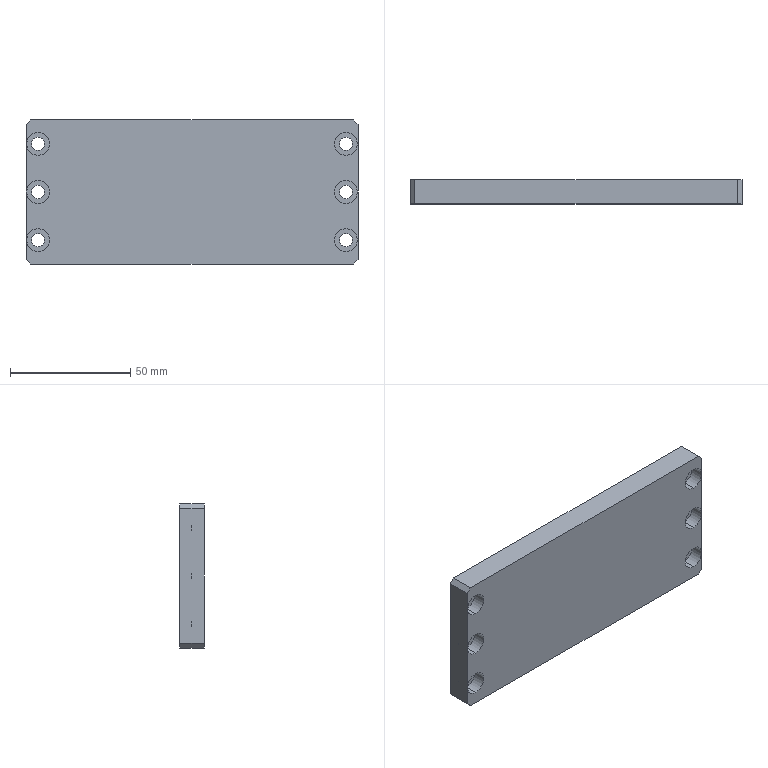Part | SolidWorks | features BaseBody 1 | 1 solid | 40 faces | box 138 x 10 x 60 mm | volume 79768 mm3 | cylinder 24 | plane 16 | commonest cylinder face diameters 5.5 x12 9.5 x12
STEP:
#1=CARTESIAN_POINT('',(-64.,5.4,-15.25));
#2=VERTEX_POINT('',#1);
#3=CARTESIAN_POINT('',(-64.,5.4,-24.75));
#4=VERTEX_POINT('',#3);
#5=CARTESIAN_POINT('',(-64.,5.4,-20.));
#6=DIRECTION('',(0.,-1.,0.));
#7=DIRECTION('',(0.,0.,-1.));
#8=AXIS2_PLACEMENT_3D('',#5,#6,#7);
#9=CIRCLE('',#8,4.75);
#10=EDGE_CURVE('',#2,#4,#9,.T.);
#11=ORIENTED_EDGE('',*,*,#10,.F.);
#12=CARTESIAN_POINT('',(-64.,0.,-15.25));
#13=VERTEX_POINT('',#12);
#14=CARTESIAN_POINT('',(-64.,0.,-15.25));
#15=DIRECTION('',(0.,-1.,0.));
#16=VECTOR('',#15,1000.);
#17=LINE('',#14,#16);
#18=EDGE_CURVE('',#2,#13,#17,.T.);
#19=ORIENTED_EDGE('',*,*,#18,.T.);
#20=CARTESIAN_POINT('',(-64.,0.,-24.75));
#21=VERTEX_POINT('',#20);
#22=CARTESIAN_POINT('',(-64.,0.,-20.));
#23=DIRECTION('',(0.,-1.,0.));
#24=DIRECTION('',(0.,0.,-1.));
#25=AXIS2_PLACEMENT_3D('',#22,#23,#24);
#26=CIRCLE('',#25,4.75);
#27=EDGE_CURVE('',#13,#21,#26,.T.);
#28=ORIENTED_EDGE('',*,*,#27,.T.);
#29=CARTESIAN_POINT('',(-64.,0.,-24.75));
#30=DIRECTION('',(0.,-1.,0.));
#31=VECTOR('',#30,1000.);
#32=LINE('',#29,#31);
#33=EDGE_CURVE('',#4,#21,#32,.T.);
#34=ORIENTED_EDGE('',*,*,#33,.F.);
#35=EDGE_LOOP('',(#11,#19,#28,#34));
#36=FACE_OUTER_BOUND('',#35,.T.);
#37=CARTESIAN_POINT('',(-64.,0.,-20.));
#38=DIRECTION('',(0.,-1.,0.));
#39=DIRECTION('',(0.,0.,-1.));
#40=AXIS2_PLACEMENT_3D('',#37,#38,#39);
#41=CYLINDRICAL_SURFACE('',#40,4.75);
#42=ADVANCED_FACE('',(#36),#41,.F.);
#43=CARTESIAN_POINT('',(-64.,10.,-17.25));
#44=VERTEX_POINT('',#43);
#45=CARTESIAN_POINT('',(-64.,10.,-22.75));
#46=VERTEX_POINT('',#45);
#47=CARTESIAN_POINT('',(-64.,10.,-20.));
#48=DIRECTION('',(0.,-1.,0.));
#49=DIRECTION('',(0.,0.,-1.));
#50=AXIS2_PLACEMENT_3D('',#47,#48,#49);
#51=CIRCLE('',#50,2.75);
#52=EDGE_CURVE('',#44,#46,#51,.T.);
#53=ORIENTED_EDGE('',*,*,#52,.F.);
#54=CARTESIAN_POINT('',(-64.,5.4,-17.25));
#55=VERTEX_POINT('',#54);
#56=CARTESIAN_POINT('',(-64.,0.,-17.25));
#57=DIRECTION('',(0.,-1.,0.));
#58=VECTOR('',#57,1000.);
#59=LINE('',#56,#58);
#60=EDGE_CURVE('',#44,#55,#59,.T.);
#61=ORIENTED_EDGE('',*,*,#60,.T.);
#62=CARTESIAN_POINT('',(-64.,5.4,-22.75));
#63=VERTEX_POINT('',#62);
#64=CARTESIAN_POINT('',(-64.,5.4,-20.));
#65=DIRECTION('',(0.,-1.,0.));
#66=DIRECTION('',(0.,0.,-1.));
#67=AXIS2_PLACEMENT_3D('',#64,#65,#66);
#68=CIRCLE('',#67,2.75);
#69=EDGE_CURVE('',#55,#63,#68,.T.);
#70=ORIENTED_EDGE('',*,*,#69,.T.);
#71=CARTESIAN_POINT('',(-64.,0.,-22.75));
#72=DIRECTION('',(0.,-1.,0.));
#73=VECTOR('',#72,1000.);
#74=LINE('',#71,#73);
#75=EDGE_CURVE('',#46,#63,#74,.T.);
#76=ORIENTED_EDGE('',*,*,#75,.F.);
#77=EDGE_LOOP('',(#53,#61,#70,#76));
#78=FACE_OUTER_BOUND('',#77,.T.);
#79=CARTESIAN_POINT('',(-64.,0.,-20.));
#80=DIRECTION('',(0.,-1.,0.));
#81=DIRECTION('',(0.,0.,-1.));
#82=AXIS2_PLACEMENT_3D('',#79,#80,#81);
#83=CYLINDRICAL_SURFACE('',#82,2.75);
#84=ADVANCED_FACE('',(#78),#83,.F.);
#85=CARTESIAN_POINT('',(-64.,5.4,4.75));
#86=VERTEX_POINT('',#85);
#87=CARTESIAN_POINT('',(-64.,5.4,-4.75));
#88=VERTEX_POINT('',#87);
#89=CARTESIAN_POINT('',(-64.,5.4,0.));
#90=DIRECTION('',(0.,-1.,0.));
#91=DIRECTION('',(0.,0.,-1.));
#92=AXIS2_PLACEMENT_3D('',#89,#90,#91);
#93=CIRCLE('',#92,4.75);
#94=EDGE_CURVE('',#86,#88,#93,.T.);
#95=ORIENTED_EDGE('',*,*,#94,.F.);
#96=CARTESIAN_POINT('',(-64.,0.,4.75));
#97=VERTEX_POINT('',#96);
#98=CARTESIAN_POINT('',(-64.,0.,4.75));
#99=DIRECTION('',(0.,-1.,0.));
#100=VECTOR('',#99,1000.);
#101=LINE('',#98,#100);
#102=EDGE_CURVE('',#86,#97,#101,.T.);
#103=ORIENTED_EDGE('',*,*,#102,.T.);
#104=CARTESIAN_POINT('',(-64.,0.,-4.75));
#105=VERTEX_POINT('',#104);
#106=CARTESIAN_POINT('',(-64.,0.,0.));
#107=DIRECTION('',(0.,-1.,0.));
#108=DIRECTION('',(0.,0.,-1.));
#109=AXIS2_PLACEMENT_3D('',#106,#107,#108);
#110=CIRCLE('',#109,4.75);
#111=EDGE_CURVE('',#97,#105,#110,.T.);
#112=ORIENTED_EDGE('',*,*,#111,.T.);
#113=CARTESIAN_POINT('',(-64.,0.,-4.75));
#114=DIRECTION('',(0.,-1.,0.));
#115=VECTOR('',#114,1000.);
#116=LINE('',#113,#115);
#117=EDGE_CURVE('',#88,#105,#116,.T.);
#118=ORIENTED_EDGE('',*,*,#117,.F.);
#119=EDGE_LOOP('',(#95,#103,#112,#118));
#120=FACE_OUTER_BOUND('',#119,.T.);
#121=CARTESIAN_POINT('',(-64.,0.,0.));
#122=DIRECTION('',(0.,-1.,0.));
#123=DIRECTION('',(0.,0.,-1.));
#124=AXIS2_PLACEMENT_3D('',#121,#122,#123);
#125=CYLINDRICAL_SURFACE('',#124,4.75);
#126=ADVANCED_FACE('',(#120),#125,.F.);
#127=CARTESIAN_POINT('',(-64.,10.,2.75));
#128=VERTEX_POINT('',#127);
#129=CARTESIAN_POINT('',(-64.,10.,-2.75));
#130=VERTEX_POINT('',#129);
#131=CARTESIAN_POINT('',(-64.,10.,0.));
#132=DIRECTION('',(0.,-1.,0.));
#133=DIRECTION('',(0.,0.,-1.));
#134=AXIS2_PLACEMENT_3D('',#131,#132,#133);
#135=CIRCLE('',#134,2.75);
#136=EDGE_CURVE('',#128,#130,#135,.T.);
#137=ORIENTED_EDGE('',*,*,#136,.F.);
#138=CARTESIAN_POINT('',(-64.,5.4,2.75));
#139=VERTEX_POINT('',#138);
#140=CARTESIAN_POINT('',(-64.,0.,2.75));
#141=DIRECTION('',(0.,-1.,0.));
#142=VECTOR('',#141,1000.);
#143=LINE('',#140,#142);
#144=EDGE_CURVE('',#128,#139,#143,.T.);
#145=ORIENTED_EDGE('',*,*,#144,.T.);
#146=CARTESIAN_POINT('',(-64.,5.4,-2.75));
#147=VERTEX_POINT('',#146);
#148=CARTESIAN_POINT('',(-64.,5.4,0.));
#149=DIRECTION('',(0.,-1.,0.));
#150=DIRECTION('',(0.,0.,-1.));
#151=AXIS2_PLACEMENT_3D('',#148,#149,#150);
#152=CIRCLE('',#151,2.75);
#153=EDGE_CURVE('',#139,#147,#152,.T.);
#154=ORIENTED_EDGE('',*,*,#153,.T.);
#155=CARTESIAN_POINT('',(-64.,0.,-2.75));
#156=DIRECTION('',(0.,-1.,0.));
#157=VECTOR('',#156,1000.);
#158=LINE('',#155,#157);
#159=EDGE_CURVE('',#130,#147,#158,.T.);
#160=ORIENTED_EDGE('',*,*,#159,.F.);
#161=EDGE_LOOP('',(#137,#145,#154,#160));
#162=FACE_OUTER_BOUND('',#161,.T.);
#163=CARTESIAN_POINT('',(-64.,0.,0.));
#164=DIRECTION('',(0.,-1.,0.));
#165=DIRECTION('',(0.,0.,-1.));
#166=AXIS2_PLACEMENT_3D('',#163,#164,#165);
#167=CYLINDRICAL_SURFACE('',#166,2.75);
#168=ADVANCED_FACE('',(#162),#167,.F.);
#169=CARTESIAN_POINT('',(-64.,5.4,24.75));
#170=VERTEX_POINT('',#169);
#171=CARTESIAN_POINT('',(-64.,5.4,15.25));
#172=VERTEX_POINT('',#171);
#173=CARTESIAN_POINT('',(-64.,5.4,20.));
#174=DIRECTION('',(0.,-1.,0.));
#175=DIRECTION('',(0.,0.,-1.));
#176=AXIS2_PLACEMENT_3D('',#173,#174,#175);
#177=CIRCLE('',#176,4.75);
#178=EDGE_CURVE('',#170,#172,#177,.T.);
#179=ORIENTED_EDGE('',*,*,#178,.F.);
#180=CARTESIAN_POINT('',(-64.,0.,24.75));
#181=VERTEX_POINT('',#180);
#182=CARTESIAN_POINT('',(-64.,0.,24.75));
#183=DIRECTION('',(0.,-1.,0.));
#184=VECTOR('',#183,1000.);
#185=LINE('',#182,#184);
#186=EDGE_CURVE('',#170,#181,#185,.T.);
#187=ORIENTED_EDGE('',*,*,#186,.T.);
#188=CARTESIAN_POINT('',(-64.,0.,15.25));
#189=VERTEX_POINT('',#188);
#190=CARTESIAN_POINT('',(-64.,0.,20.));
#191=DIRECTION('',(0.,-1.,0.));
#192=DIRECTION('',(0.,0.,-1.));
#193=AXIS2_PLACEMENT_3D('',#190,#191,#192);
#194=CIRCLE('',#193,4.75);
#195=EDGE_CURVE('',#181,#189,#194,.T.);
#196=ORIENTED_EDGE('',*,*,#195,.T.);
#197=CARTESIAN_POINT('',(-64.,0.,15.25));
#198=DIRECTION('',(0.,-1.,0.));
#199=VECTOR('',#198,1000.);
#200=LINE('',#197,#199);
#201=EDGE_CURVE('',#172,#189,#200,.T.);
#202=ORIENTED_EDGE('',*,*,#201,.F.);
#203=EDGE_LOOP('',(#179,#187,#196,#202));
#204=FACE_OUTER_BOUND('',#203,.T.);
#205=CARTESIAN_POINT('',(-64.,0.,20.));
#206=DIRECTION('',(0.,-1.,0.));
#207=DIRECTION('',(0.,0.,-1.));
#208=AXIS2_PLACEMENT_3D('',#205,#206,#207);
#209=CYLINDRICAL_SURFACE('',#208,4.75);
#210=ADVANCED_FACE('',(#204),#209,.F.);
#211=CARTESIAN_POINT('',(-64.,10.,22.75));
#212=VERTEX_POINT('',#211);
#213=CARTESIAN_POINT('',(-64.,10.,17.25));
#214=VERTEX_POINT('',#213);
#215=CARTESIAN_POINT('',(-64.,10.,20.));
#216=DIRECTION('',(0.,-1.,0.));
#217=DIRECTION('',(0.,0.,-1.));
#218=AXIS2_PLACEMENT_3D('',#215,#216,#217);
#219=CIRCLE('',#218,2.75);
#220=EDGE_CURVE('',#212,#214,#219,.T.);
#221=ORIENTED_EDGE('',*,*,#220,.F.);
#222=CARTESIAN_POINT('',(-64.,5.4,22.75));
#223=VERTEX_POINT('',#222);
#224=CARTESIAN_POINT('',(-64.,0.,22.75));
#225=DIRECTION('',(0.,-1.,0.));
#226=VECTOR('',#225,1000.);
#227=LINE('',#224,#226);
#228=EDGE_CURVE('',#212,#223,#227,.T.);
#229=ORIENTED_EDGE('',*,*,#228,.T.);
#230=CARTESIAN_POINT('',(-64.,5.4,17.25));
#231=VERTEX_POINT('',#230);
#232=CARTESIAN_POINT('',(-64.,5.4,20.));
#233=DIRECTION('',(0.,-1.,0.));
#234=DIRECTION('',(0.,0.,-1.));
#235=AXIS2_PLACEMENT_3D('',#232,#233,#234);
#236=CIRCLE('',#235,2.75);
#237=EDGE_CURVE('',#223,#231,#236,.T.);
#238=ORIENTED_EDGE('',*,*,#237,.T.);
#239=CARTESIAN_POINT('',(-64.,0.,17.25));
#240=DIRECTION('',(0.,-1.,0.));
#241=VECTOR('',#240,1000.);
#242=LINE('',#239,#241);
#243=EDGE_CURVE('',#214,#231,#242,.T.);
#244=ORIENTED_EDGE('',*,*,#243,.F.);
#245=EDGE_LOOP('',(#221,#229,#238,#244));
#246=FACE_OUTER_BOUND('',#245,.T.);
#247=CARTESIAN_POINT('',(-64.,0.,20.));
#248=DIRECTION('',(0.,-1.,0.));
#249=DIRECTION('',(0.,0.,-1.));
#250=AXIS2_PLACEMENT_3D('',#247,#248,#249);
#251=CYLINDRICAL_SURFACE('',#250,2.75);
#252=ADVANCED_FACE('',(#246),#251,.F.);
#253=CARTESIAN_POINT('',(64.,5.4,24.75));
#254=VERTEX_POINT('',#253);
#255=CARTESIAN_POINT('',(64.,5.4,15.25));
#256=VERTEX_POINT('',#255);
#257=CARTESIAN_POINT('',(64.,5.4,20.));
#258=DIRECTION('',(0.,-1.,0.));
#259=DIRECTION('',(0.,0.,-1.));
#260=AXIS2_PLACEMENT_3D('',#257,#258,#259);
#261=CIRCLE('',#260,4.75);
#262=EDGE_CURVE('',#254,#256,#261,.T.);
#263=ORIENTED_EDGE('',*,*,#262,.F.);
#264=CARTESIAN_POINT('',(64.,0.,24.75));
#265=VERTEX_POINT('',#264);
#266=CARTESIAN_POINT('',(64.,0.,24.75));
#267=DIRECTION('',(0.,-1.,0.));
#268=VECTOR('',#267,1000.);
#269=LINE('',#266,#268);
#270=EDGE_CURVE('',#254,#265,#269,.T.);
#271=ORIENTED_EDGE('',*,*,#270,.T.);
#272=CARTESIAN_POINT('',(64.,0.,15.25));
#273=VERTEX_POINT('',#272);
#274=CARTESIAN_POINT('',(64.,0.,20.));
#275=DIRECTION('',(0.,-1.,0.));
#276=DIRECTION('',(0.,0.,-1.));
#277=AXIS2_PLACEMENT_3D('',#274,#275,#276);
#278=CIRCLE('',#277,4.75);
#279=EDGE_CURVE('',#265,#273,#278,.T.);
#280=ORIENTED_EDGE('',*,*,#279,.T.);
#281=CARTESIAN_POINT('',(64.,0.,15.25));
#282=DIRECTION('',(0.,-1.,0.));
#283=VECTOR('',#282,1000.);
#284=LINE('',#281,#283);
#285=EDGE_CURVE('',#256,#273,#284,.T.);
#286=ORIENTED_EDGE('',*,*,#285,.F.);
#287=EDGE_LOOP('',(#263,#271,#280,#286));
#288=FACE_OUTER_BOUND('',#287,.T.);
#289=CARTESIAN_POINT('',(64.,0.,20.));
#290=DIRECTION('',(0.,-1.,0.));
#291=DIRECTION('',(0.,0.,-1.));
#292=AXIS2_PLACEMENT_3D('',#289,#290,#291);
#293=CYLINDRICAL_SURFACE('',#292,4.75);
#294=ADVANCED_FACE('',(#288),#293,.F.);
#295=CARTESIAN_POINT('',(64.,10.,22.75));
#296=VERTEX_POINT('',#295);
#297=CARTESIAN_POINT('',(64.,10.,17.25));
#298=VERTEX_POINT('',#297);
#299=CARTESIAN_POINT('',(64.,10.,20.));
#300=DIRECTION('',(0.,-1.,0.));
#301=DIRECTION('',(0.,0.,-1.));
#302=AXIS2_PLACEMENT_3D('',#299,#300,#301);
#303=CIRCLE('',#302,2.75);
#304=EDGE_CURVE('',#296,#298,#303,.T.);
#305=ORIENTED_EDGE('',*,*,#304,.F.);
#306=CARTESIAN_POINT('',(64.,5.4,22.75));
#307=VERTEX_POINT('',#306);
#308=CARTESIAN_POINT('',(64.,0.,22.75));
#309=DIRECTION('',(0.,-1.,0.));
#310=VECTOR('',#309,1000.);
#311=LINE('',#308,#310);
#312=EDGE_CURVE('',#296,#307,#311,.T.);
#313=ORIENTED_EDGE('',*,*,#312,.T.);
#314=CARTESIAN_POINT('',(64.,5.4,17.25));
#315=VERTEX_POINT('',#314);
#316=CARTESIAN_POINT('',(64.,5.4,20.));
#317=DIRECTION('',(0.,-1.,0.));
#318=DIRECTION('',(0.,0.,-1.));
#319=AXIS2_PLACEMENT_3D('',#316,#317,#318);
#320=CIRCLE('',#319,2.75);
#321=EDGE_CURVE('',#307,#315,#320,.T.);
#322=ORIENTED_EDGE('',*,*,#321,.T.);
#323=CARTESIAN_POINT('',(64.,0.,17.25));
#324=DIRECTION('',(0.,-1.,0.));
#325=VECTOR('',#324,1000.);
#326=LINE('',#323,#325);
#327=EDGE_CURVE('',#298,#315,#326,.T.);
#328=ORIENTED_EDGE('',*,*,#327,.F.);
#329=EDGE_LOOP('',(#305,#313,#322,#328));
#330=FACE_OUTER_BOUND('',#329,.T.);
#331=CARTESIAN_POINT('',(64.,0.,20.));
#332=DIRECTION('',(0.,-1.,0.));
#333=DIRECTION('',(0.,0.,-1.));
#334=AXIS2_PLACEMENT_3D('',#331,#332,#333);
#335=CYLINDRICAL_SURFACE('',#334,2.75);
#336=ADVANCED_FACE('',(#330),#335,.F.);
#337=CARTESIAN_POINT('',(64.,5.4,4.75));
#338=VERTEX_POINT('',#337);
#339=CARTESIAN_POINT('',(64.,5.4,-4.75));
#340=VERTEX_POINT('',#339);
#341=CARTESIAN_POINT('',(64.,5.4,0.));
#342=DIRECTION('',(0.,-1.,0.));
#343=DIRECTION('',(0.,0.,-1.));
#344=AXIS2_PLACEMENT_3D('',#341,#342,#343);
#345=CIRCLE('',#344,4.75);
#346=EDGE_CURVE('',#338,#340,#345,.T.);
#347=ORIENTED_EDGE('',*,*,#346,.F.);
#348=CARTESIAN_POINT('',(64.,0.,4.75));
#349=VERTEX_POINT('',#348);
#350=CARTESIAN_POINT('',(64.,0.,4.75));
#351=DIRECTION('',(0.,-1.,0.));
#352=VECTOR('',#351,1000.);
#353=LINE('',#350,#352);
#354=EDGE_CURVE('',#338,#349,#353,.T.);
#355=ORIENTED_EDGE('',*,*,#354,.T.);
#356=CARTESIAN_POINT('',(64.,0.,-4.75));
#357=VERTEX_POINT('',#356);
#358=CARTESIAN_POINT('',(64.,0.,0.));
#359=DIRECTION('',(0.,-1.,0.));
#360=DIRECTION('',(0.,0.,-1.));
#361=AXIS2_PLACEMENT_3D('',#358,#359,#360);
#362=CIRCLE('',#361,4.75);
#363=EDGE_CURVE('',#349,#357,#362,.T.);
#364=ORIENTED_EDGE('',*,*,#363,.T.);
#365=CARTESIAN_POINT('',(64.,0.,-4.75));
#366=DIRECTION('',(0.,-1.,0.));
#367=VECTOR('',#366,1000.);
#368=LINE('',#365,#367);
#369=EDGE_CURVE('',#340,#357,#368,.T.);
#370=ORIENTED_EDGE('',*,*,#369,.F.);
#371=EDGE_LOOP('',(#347,#355,#364,#370));
#372=FACE_OUTER_BOUND('',#371,.T.);
#373=CARTESIAN_POINT('',(64.,0.,0.));
#374=DIRECTION('',(0.,-1.,0.));
#375=DIRECTION('',(0.,0.,-1.));
#376=AXIS2_PLACEMENT_3D('',#373,#374,#375);
#377=CYLINDRICAL_SURFACE('',#376,4.75);
#378=ADVANCED_FACE('',(#372),#377,.F.);
#379=CARTESIAN_POINT('',(64.,10.,2.75));
#380=VERTEX_POINT('',#379);
#381=CARTESIAN_POINT('',(64.,10.,-2.75));
#382=VERTEX_POINT('',#381);
#383=CARTESIAN_POINT('',(64.,10.,0.));
#384=DIRECTION('',(0.,-1.,0.));
#385=DIRECTION('',(0.,0.,-1.));
#386=AXIS2_PLACEMENT_3D('',#383,#384,#385);
#387=CIRCLE('',#386,2.75);
#388=EDGE_CURVE('',#380,#382,#387,.T.);
#389=ORIENTED_EDGE('',*,*,#388,.F.);
#390=CARTESIAN_POINT('',(64.,5.4,2.75));
#391=VERTEX_POINT('',#390);
#392=CARTESIAN_POINT('',(64.,0.,2.75));
#393=DIRECTION('',(0.,-1.,0.));
#394=VECTOR('',#393,1000.);
#395=LINE('',#392,#394);
#396=EDGE_CURVE('',#380,#391,#395,.T.);
#397=ORIENTED_EDGE('',*,*,#396,.T.);
#398=CARTESIAN_POINT('',(64.,5.4,-2.75));
#399=VERTEX_POINT('',#398);
#400=CARTESIAN_POINT('',(64.,5.4,0.));
#401=DIRECTION('',(0.,-1.,0.));
#402=DIRECTION('',(0.,0.,-1.));
#403=AXIS2_PLACEMENT_3D('',#400,#401,#402);
#404=CIRCLE('',#403,2.75);
#405=EDGE_CURVE('',#391,#399,#404,.T.);
#406=ORIENTED_EDGE('',*,*,#405,.T.);
#407=CARTESIAN_POINT('',(64.,0.,-2.75));
#408=DIRECTION('',(0.,-1.,0.));
#409=VECTOR('',#408,1000.);
#410=LINE('',#407,#409);
#411=EDGE_CURVE('',#382,#399,#410,.T.);
#412=ORIENTED_EDGE('',*,*,#411,.F.);
#413=EDGE_LOOP('',(#389,#397,#406,#412));
#414=FACE_OUTER_BOUND('',#413,.T.);
#415=CARTESIAN_POINT('',(64.,0.,0.));
#416=DIRECTION('',(0.,-1.,0.));
#417=DIRECTION('',(0.,0.,-1.));
#418=AXIS2_PLACEMENT_3D('',#415,#416,#417);
#419=CYLINDRICAL_SURFACE('',#418,2.75);
#420=ADVANCED_FACE('',(#414),#419,.F.);
#421=CARTESIAN_POINT('',(64.,5.4,-15.25));
#422=VERTEX_POINT('',#421);
#423=CARTESIAN_POINT('',(64.,5.4,-24.75));
#424=VERTEX_POINT('',#423);
#425=CARTESIAN_POINT('',(64.,5.4,-20.));
#426=DIRECTION('',(0.,-1.,0.));
#427=DIRECTION('',(0.,0.,-1.));
#428=AXIS2_PLACEMENT_3D('',#425,#426,#427);
#429=CIRCLE('',#428,4.75);
#430=EDGE_CURVE('',#422,#424,#429,.T.);
#431=ORIENTED_EDGE('',*,*,#430,.F.);
#432=CARTESIAN_POINT('',(64.,0.,-15.25));
#433=VERTEX_POINT('',#432);
#434=CARTESIAN_POINT('',(64.,0.,-15.25));
#435=DIRECTION('',(0.,-1.,0.));
#436=VECTOR('',#435,1000.);
#437=LINE('',#434,#436);
#438=EDGE_CURVE('',#422,#433,#437,.T.);
#439=ORIENTED_EDGE('',*,*,#438,.T.);
#440=CARTESIAN_POINT('',(64.,0.,-24.75));
#441=VERTEX_POINT('',#440);
#442=CARTESIAN_POINT('',(64.,0.,-20.));
#443=DIRECTION('',(0.,-1.,0.));
#444=DIRECTION('',(0.,0.,-1.));
#445=AXIS2_PLACEMENT_3D('',#442,#443,#444);
#446=CIRCLE('',#445,4.75);
#447=EDGE_CURVE('',#433,#441,#446,.T.);
#448=ORIENTED_EDGE('',*,*,#447,.T.);
#449=CARTESIAN_POINT('',(64.,0.,-24.75));
#450=DIRECTION('',(0.,-1.,0.));
#451=VECTOR('',#450,1000.);
#452=LINE('',#449,#451);
#453=EDGE_CURVE('',#424,#441,#452,.T.);
#454=ORIENTED_EDGE('',*,*,#453,.F.);
#455=EDGE_LOOP('',(#431,#439,#448,#454));
#456=FACE_OUTER_BOUND('',#455,.T.);
#457=CARTESIAN_POINT('',(64.,0.,-20.));
#458=DIRECTION('',(0.,-1.,0.));
#459=DIRECTION('',(0.,0.,-1.));
#460=AXIS2_PLACEMENT_3D('',#457,#458,#459);
#461=CYLINDRICAL_SURFACE('',#460,4.75);
#462=ADVANCED_FACE('',(#456),#461,.F.);
#463=CARTESIAN_POINT('',(64.,10.,-17.25));
#464=VERTEX_POINT('',#463);
#465=CARTESIAN_POINT('',(64.,10.,-22.75));
#466=VERTEX_POINT('',#465);
#467=CARTESIAN_POINT('',(64.,10.,-20.));
#468=DIRECTION('',(0.,-1.,0.));
#469=DIRECTION('',(0.,0.,-1.));
#470=AXIS2_PLACEMENT_3D('',#467,#468,#469);
#471=CIRCLE('',#470,2.75);
#472=EDGE_CURVE('',#464,#466,#471,.T.);
#473=ORIENTED_EDGE('',*,*,#472,.F.);
#474=CARTESIAN_POINT('',(64.,5.4,-17.25));
#475=VERTEX_POINT('',#474);
#476=CARTESIAN_POINT('',(64.,0.,-17.25));
#477=DIRECTION('',(0.,-1.,0.));
#478=VECTOR('',#477,1000.);
#479=LINE('',#476,#478);
#480=EDGE_CURVE('',#464,#475,#479,.T.);
#481=ORIENTED_EDGE('',*,*,#480,.T.);
#482=CARTESIAN_POINT('',(64.,5.4,-22.75));
#483=VERTEX_POINT('',#482);
#484=CARTESIAN_POINT('',(64.,5.4,-20.));
#485=DIRECTION('',(0.,-1.,0.));
#486=DIRECTION('',(0.,0.,-1.));
#487=AXIS2_PLACEMENT_3D('',#484,#485,#486);
#488=CIRCLE('',#487,2.75);
#489=EDGE_CURVE('',#475,#483,#488,.T.);
#490=ORIENTED_EDGE('',*,*,#489,.T.);
#491=CARTESIAN_POINT('',(64.,0.,-22.75));
#492=DIRECTION('',(0.,-1.,0.));
#493=VECTOR('',#492,1000.);
#494=LINE('',#491,#493);
#495=EDGE_CURVE('',#466,#483,#494,.T.);
#496=ORIENTED_EDGE('',*,*,#495,.F.);
#497=EDGE_LOOP('',(#473,#481,#490,#496));
#498=FACE_OUTER_BOUND('',#497,.T.);
#499=CARTESIAN_POINT('',(64.,0.,-20.));
#500=DIRECTION('',(0.,-1.,0.));
#501=DIRECTION('',(0.,0.,-1.));
#502=AXIS2_PLACEMENT_3D('',#499,#500,#501);
#503=CYLINDRICAL_SURFACE('',#502,2.75);
#504=ADVANCED_FACE('',(#498),#503,.F.);
#505=CARTESIAN_POINT('',(-69.,10.,-28.));
#506=VERTEX_POINT('',#505);
#507=CARTESIAN_POINT('',(-69.,10.,28.));
#508=VERTEX_POINT('',#507);
#509=CARTESIAN_POINT('',(-69.,10.,-30.));
#510=DIRECTION('',(0.,0.,1.));
#511=VECTOR('',#510,1000.);
#512=LINE('',#509,#511);
#513=EDGE_CURVE('',#506,#508,#512,.T.);
#514=ORIENTED_EDGE('',*,*,#513,.F.);
#515=CARTESIAN_POINT('',(-69.,0.,-28.));
#516=VERTEX_POINT('',#515);
#517=CARTESIAN_POINT('',(-69.,10.,-28.));
#518=DIRECTION('',(0.,-1.,0.));
#519=VECTOR('',#518,1000.);
#520=LINE('',#517,#519);
#521=EDGE_CURVE('',#506,#516,#520,.T.);
#522=ORIENTED_EDGE('',*,*,#521,.T.);
#523=CARTESIAN_POINT('',(-69.,0.,28.));
#524=VERTEX_POINT('',#523);
#525=CARTESIAN_POINT('',(-69.,0.,-30.));
#526=DIRECTION('',(0.,0.,1.));
#527=VECTOR('',#526,1000.);
#528=LINE('',#525,#527);
#529=EDGE_CURVE('',#516,#524,#528,.T.);
#530=ORIENTED_EDGE('',*,*,#529,.T.);
#531=CARTESIAN_POINT('',(-69.,10.,28.));
#532=DIRECTION('',(0.,1.,0.));
#533=VECTOR('',#532,1000.);
#534=LINE('',#531,#533);
#535=EDGE_CURVE('',#524,#508,#534,.T.);
#536=ORIENTED_EDGE('',*,*,#535,.T.);
#537=EDGE_LOOP('',(#514,#522,#530,#536));
#538=FACE_OUTER_BOUND('',#537,.T.);
#539=CARTESIAN_POINT('',(-69.,10.,-30.));
#540=DIRECTION('',(1.,0.,0.));
#541=DIRECTION('',(0.,0.,-1.));
#542=AXIS2_PLACEMENT_3D('',#539,#540,#541);
#543=PLANE('',#542);
#544=ADVANCED_FACE('',(#538),#543,.F.);
#545=CARTESIAN_POINT('',(-67.,0.,30.));
#546=VERTEX_POINT('',#545);
#547=CARTESIAN_POINT('',(67.,0.,30.));
#548=VERTEX_POINT('',#547);
#549=CARTESIAN_POINT('',(69.,0.,30.));
#550=DIRECTION('',(1.,0.,0.));
#551=VECTOR('',#550,1000.);
#552=LINE('',#549,#551);
#553=EDGE_CURVE('',#546,#548,#552,.T.);
#554=ORIENTED_EDGE('',*,*,#553,.T.);
#555=CARTESIAN_POINT('',(67.,10.,30.));
#556=VERTEX_POINT('',#555);
#557=CARTESIAN_POINT('',(67.,10.,30.));
#558=DIRECTION('',(0.,1.,0.));
#559=VECTOR('',#558,1000.);
#560=LINE('',#557,#559);
#561=EDGE_CURVE('',#548,#556,#560,.T.);
#562=ORIENTED_EDGE('',*,*,#561,.T.);
#563=CARTESIAN_POINT('',(-67.,10.,30.));
#564=VERTEX_POINT('',#563);
#565=CARTESIAN_POINT('',(69.,10.,30.));
#566=DIRECTION('',(1.,0.,0.));
#567=VECTOR('',#566,1000.);
#568=LINE('',#565,#567);
#569=EDGE_CURVE('',#564,#556,#568,.T.);
#570=ORIENTED_EDGE('',*,*,#569,.F.);
#571=CARTESIAN_POINT('',(-67.,10.,30.));
#572=DIRECTION('',(0.,-1.,0.));
#573=VECTOR('',#572,1000.);
#574=LINE('',#571,#573);
#575=EDGE_CURVE('',#564,#546,#574,.T.);
#576=ORIENTED_EDGE('',*,*,#575,.T.);
#577=EDGE_LOOP('',(#554,#562,#570,#576));
#578=FACE_OUTER_BOUND('',#577,.T.);
#579=CARTESIAN_POINT('',(69.,10.,30.));
#580=DIRECTION('',(0.,0.,-1.));
#581=DIRECTION('',(-1.,0.,0.));
#582=AXIS2_PLACEMENT_3D('',#579,#580,#581);
#583=PLANE('',#582);
#584=ADVANCED_FACE('',(#578),#583,.F.);
#585=CARTESIAN_POINT('',(69.,10.,28.));
#586=VERTEX_POINT('',#585);
#587=CARTESIAN_POINT('',(69.,10.,-28.));
#588=VERTEX_POINT('',#587);
#589=CARTESIAN_POINT('',(69.,10.,-30.));
#590=DIRECTION('',(0.,0.,-1.));
#591=VECTOR('',#590,1000.);
#592=LINE('',#589,#591);
#593=EDGE_CURVE('',#586,#588,#592,.T.);
#594=ORIENTED_EDGE('',*,*,#593,.F.);
#595=CARTESIAN_POINT('',(69.,0.,28.));
#596=VERTEX_POINT('',#595);
#597=CARTESIAN_POINT('',(69.,10.,28.));
#598=DIRECTION('',(0.,-1.,0.));
#599=VECTOR('',#598,1000.);
#600=LINE('',#597,#599);
#601=EDGE_CURVE('',#586,#596,#600,.T.);
#602=ORIENTED_EDGE('',*,*,#601,.T.);
#603=CARTESIAN_POINT('',(69.,0.,-28.));
#604=VERTEX_POINT('',#603);
#605=CARTESIAN_POINT('',(69.,0.,-30.));
#606=DIRECTION('',(0.,0.,-1.));
#607=VECTOR('',#606,1000.);
#608=LINE('',#605,#607);
#609=EDGE_CURVE('',#596,#604,#608,.T.);
#610=ORIENTED_EDGE('',*,*,#609,.T.);
#611=CARTESIAN_POINT('',(69.,10.,-28.));
#612=DIRECTION('',(0.,1.,0.));
#613=VECTOR('',#612,1000.);
#614=LINE('',#611,#613);
#615=EDGE_CURVE('',#604,#588,#614,.T.);
#616=ORIENTED_EDGE('',*,*,#615,.T.);
#617=EDGE_LOOP('',(#594,#602,#610,#616));
#618=FACE_OUTER_BOUND('',#617,.T.);
#619=CARTESIAN_POINT('',(69.,10.,-30.));
#620=DIRECTION('',(-1.,0.,0.));
#621=DIRECTION('',(0.,0.,1.));
#622=AXIS2_PLACEMENT_3D('',#619,#620,#621);
#623=PLANE('',#622);
#624=ADVANCED_FACE('',(#618),#623,.F.);
#625=CARTESIAN_POINT('',(67.,10.,-30.));
#626=VERTEX_POINT('',#625);
#627=CARTESIAN_POINT('',(-67.,10.,-30.));
#628=VERTEX_POINT('',#627);
#629=CARTESIAN_POINT('',(69.,10.,-30.));
#630=DIRECTION('',(-1.,0.,0.));
#631=VECTOR('',#630,1000.);
#632=LINE('',#629,#631);
#633=EDGE_CURVE('',#626,#628,#632,.T.);
#634=ORIENTED_EDGE('',*,*,#633,.F.);
#635=CARTESIAN_POINT('',(67.,0.,-30.));
#636=VERTEX_POINT('',#635);
#637=CARTESIAN_POINT('',(67.,10.,-30.));
#638=DIRECTION('',(0.,-1.,0.));
#639=VECTOR('',#638,1000.);
#640=LINE('',#637,#639);
#641=EDGE_CURVE('',#626,#636,#640,.T.);
#642=ORIENTED_EDGE('',*,*,#641,.T.);
#643=CARTESIAN_POINT('',(-67.,0.,-30.));
#644=VERTEX_POINT('',#643);
#645=CARTESIAN_POINT('',(69.,0.,-30.));
#646=DIRECTION('',(-1.,0.,0.));
#647=VECTOR('',#646,1000.);
#648=LINE('',#645,#647);
#649=EDGE_CURVE('',#636,#644,#648,.T.);
#650=ORIENTED_EDGE('',*,*,#649,.T.);
#651=CARTESIAN_POINT('',(-67.,10.,-30.));
#652=DIRECTION('',(0.,1.,0.));
#653=VECTOR('',#652,1000.);
#654=LINE('',#651,#653);
#655=EDGE_CURVE('',#644,#628,#654,.T.);
#656=ORIENTED_EDGE('',*,*,#655,.T.);
#657=EDGE_LOOP('',(#634,#642,#650,#656));
#658=FACE_OUTER_BOUND('',#657,.T.);
#659=CARTESIAN_POINT('',(69.,10.,-30.));
#660=DIRECTION('',(0.,0.,1.));
#661=DIRECTION('',(1.,0.,0.));
#662=AXIS2_PLACEMENT_3D('',#659,#660,#661);
#663=PLANE('',#662);
#664=ADVANCED_FACE('',(#658),#663,.F.);
#665=CARTESIAN_POINT('',(-64.,10.,-20.));
#666=DIRECTION('',(0.,-1.,0.));
#667=DIRECTION('',(0.,0.,-1.));
#668=AXIS2_PLACEMENT_3D('',#665,#666,#667);
#669=CIRCLE('',#668,2.75);
#670=EDGE_CURVE('',#46,#44,#669,.T.);
#671=ORIENTED_EDGE('',*,*,#670,.T.);
#672=ORIENTED_EDGE('',*,*,#52,.T.);
#673=EDGE_LOOP('',(#671,#672));
#674=FACE_BOUND('',#673,.T.);
#675=CARTESIAN_POINT('',(-64.,10.,0.));
#676=DIRECTION('',(0.,-1.,0.));
#677=DIRECTION('',(0.,0.,-1.));
#678=AXIS2_PLACEMENT_3D('',#675,#676,#677);
#679=CIRCLE('',#678,2.75);
#680=EDGE_CURVE('',#130,#128,#679,.T.);
#681=ORIENTED_EDGE('',*,*,#680,.T.);
#682=ORIENTED_EDGE('',*,*,#136,.T.);
#683=EDGE_LOOP('',(#681,#682));
#684=FACE_BOUND('',#683,.T.);
#685=CARTESIAN_POINT('',(-64.,10.,20.));
#686=DIRECTION('',(0.,-1.,0.));
#687=DIRECTION('',(0.,0.,-1.));
#688=AXIS2_PLACEMENT_3D('',#685,#686,#687);
#689=CIRCLE('',#688,2.75);
#690=EDGE_CURVE('',#214,#212,#689,.T.);
#691=ORIENTED_EDGE('',*,*,#690,.T.);
#692=ORIENTED_EDGE('',*,*,#220,.T.);
#693=EDGE_LOOP('',(#691,#692));
#694=FACE_BOUND('',#693,.T.);
#695=CARTESIAN_POINT('',(64.,10.,20.));
#696=DIRECTION('',(0.,-1.,0.));
#697=DIRECTION('',(0.,0.,-1.));
#698=AXIS2_PLACEMENT_3D('',#695,#696,#697);
#699=CIRCLE('',#698,2.75);
#700=EDGE_CURVE('',#298,#296,#699,.T.);
#701=ORIENTED_EDGE('',*,*,#700,.T.);
#702=ORIENTED_EDGE('',*,*,#304,.T.);
#703=EDGE_LOOP('',(#701,#702));
#704=FACE_BOUND('',#703,.T.);
#705=CARTESIAN_POINT('',(64.,10.,0.));
#706=DIRECTION('',(0.,-1.,0.));
#707=DIRECTION('',(0.,0.,-1.));
#708=AXIS2_PLACEMENT_3D('',#705,#706,#707);
#709=CIRCLE('',#708,2.75);
#710=EDGE_CURVE('',#382,#380,#709,.T.);
#711=ORIENTED_EDGE('',*,*,#710,.T.);
#712=ORIENTED_EDGE('',*,*,#388,.T.);
#713=EDGE_LOOP('',(#711,#712));
#714=FACE_BOUND('',#713,.T.);
#715=CARTESIAN_POINT('',(64.,10.,-20.));
#716=DIRECTION('',(0.,-1.,0.));
#717=DIRECTION('',(0.,0.,-1.));
#718=AXIS2_PLACEMENT_3D('',#715,#716,#717);
#719=CIRCLE('',#718,2.75);
#720=EDGE_CURVE('',#466,#464,#719,.T.);
#721=ORIENTED_EDGE('',*,*,#720,.T.);
#722=ORIENTED_EDGE('',*,*,#472,.T.);
#723=EDGE_LOOP('',(#721,#722));
#724=FACE_BOUND('',#723,.T.);
#725=ORIENTED_EDGE('',*,*,#569,.T.);
#726=CARTESIAN_POINT('',(69.,10.,28.));
#727=DIRECTION('',(0.7071,0.,-0.7071));
#728=VECTOR('',#727,1000.);
#729=LINE('',#726,#728);
#730=EDGE_CURVE('',#556,#586,#729,.T.);
#731=ORIENTED_EDGE('',*,*,#730,.T.);
#732=ORIENTED_EDGE('',*,*,#593,.T.);
#733=CARTESIAN_POINT('',(67.,10.,-30.));
#734=DIRECTION('',(-0.7071,0.,-0.7071));
#735=VECTOR('',#734,1000.);
#736=LINE('',#733,#735);
#737=EDGE_CURVE('',#588,#626,#736,.T.);
#738=ORIENTED_EDGE('',*,*,#737,.T.);
#739=ORIENTED_EDGE('',*,*,#633,.T.);
#740=CARTESIAN_POINT('',(-69.,10.,-28.));
#741=DIRECTION('',(-0.7071,0.,0.7071));
#742=VECTOR('',#741,1000.);
#743=LINE('',#740,#742);
#744=EDGE_CURVE('',#628,#506,#743,.T.);
#745=ORIENTED_EDGE('',*,*,#744,.T.);
#746=ORIENTED_EDGE('',*,*,#513,.T.);
#747=CARTESIAN_POINT('',(-67.,10.,30.));
#748=DIRECTION('',(0.7071,0.,0.7071));
#749=VECTOR('',#748,1000.);
#750=LINE('',#747,#749);
#751=EDGE_CURVE('',#508,#564,#750,.T.);
#752=ORIENTED_EDGE('',*,*,#751,.T.);
#753=EDGE_LOOP('',(#725,#731,#732,#738,#739,#745,#746,#752));
#754=FACE_OUTER_BOUND('',#753,.T.);
#755=CARTESIAN_POINT('',(0.,10.,0.));
#756=DIRECTION('',(0.,-1.,0.));
#757=DIRECTION('',(0.,0.,-1.));
#758=AXIS2_PLACEMENT_3D('',#755,#756,#757);
#759=PLANE('',#758);
#760=ADVANCED_FACE('',(#674,#684,#694,#704,#714,#724,#754),#759,.F.);
#761=CARTESIAN_POINT('',(-64.,0.,-20.));
#762=DIRECTION('',(0.,-1.,0.));
#763=DIRECTION('',(0.,0.,-1.));
#764=AXIS2_PLACEMENT_3D('',#761,#762,#763);
#765=CIRCLE('',#764,4.75);
#766=EDGE_CURVE('',#21,#13,#765,.T.);
#767=ORIENTED_EDGE('',*,*,#766,.F.);
#768=ORIENTED_EDGE('',*,*,#27,.F.);
#769=EDGE_LOOP('',(#767,#768));
#770=FACE_BOUND('',#769,.T.);
#771=CARTESIAN_POINT('',(-64.,0.,0.));
#772=DIRECTION('',(0.,-1.,0.));
#773=DIRECTION('',(0.,0.,-1.));
#774=AXIS2_PLACEMENT_3D('',#771,#772,#773);
#775=CIRCLE('',#774,4.75);
#776=EDGE_CURVE('',#105,#97,#775,.T.);
#777=ORIENTED_EDGE('',*,*,#776,.F.);
#778=ORIENTED_EDGE('',*,*,#111,.F.);
#779=EDGE_LOOP('',(#777,#778));
#780=FACE_BOUND('',#779,.T.);
#781=CARTESIAN_POINT('',(-64.,0.,20.));
#782=DIRECTION('',(0.,-1.,0.));
#783=DIRECTION('',(0.,0.,-1.));
#784=AXIS2_PLACEMENT_3D('',#781,#782,#783);
#785=CIRCLE('',#784,4.75);
#786=EDGE_CURVE('',#189,#181,#785,.T.);
#787=ORIENTED_EDGE('',*,*,#786,.F.);
#788=ORIENTED_EDGE('',*,*,#195,.F.);
#789=EDGE_LOOP('',(#787,#788));
#790=FACE_BOUND('',#789,.T.);
#791=CARTESIAN_POINT('',(64.,0.,20.));
#792=DIRECTION('',(0.,-1.,0.));
#793=DIRECTION('',(0.,0.,-1.));
#794=AXIS2_PLACEMENT_3D('',#791,#792,#793);
#795=CIRCLE('',#794,4.75);
#796=EDGE_CURVE('',#273,#265,#795,.T.);
#797=ORIENTED_EDGE('',*,*,#796,.F.);
#798=ORIENTED_EDGE('',*,*,#279,.F.);
#799=EDGE_LOOP('',(#797,#798));
#800=FACE_BOUND('',#799,.T.);
#801=CARTESIAN_POINT('',(64.,0.,0.));
#802=DIRECTION('',(0.,-1.,0.));
#803=DIRECTION('',(0.,0.,-1.));
#804=AXIS2_PLACEMENT_3D('',#801,#802,#803);
#805=CIRCLE('',#804,4.75);
#806=EDGE_CURVE('',#357,#349,#805,.T.);
#807=ORIENTED_EDGE('',*,*,#806,.F.);
#808=ORIENTED_EDGE('',*,*,#363,.F.);
#809=EDGE_LOOP('',(#807,#808));
#810=FACE_BOUND('',#809,.T.);
#811=CARTESIAN_POINT('',(64.,0.,-20.));
#812=DIRECTION('',(0.,-1.,0.));
#813=DIRECTION('',(0.,0.,-1.));
#814=AXIS2_PLACEMENT_3D('',#811,#812,#813);
#815=CIRCLE('',#814,4.75);
#816=EDGE_CURVE('',#441,#433,#815,.T.);
#817=ORIENTED_EDGE('',*,*,#816,.F.);
#818=ORIENTED_EDGE('',*,*,#447,.F.);
#819=EDGE_LOOP('',(#817,#818));
#820=FACE_BOUND('',#819,.T.);
#821=ORIENTED_EDGE('',*,*,#609,.F.);
#822=CARTESIAN_POINT('',(48.5,0.,48.5));
#823=DIRECTION('',(-0.7071,0.,0.7071));
#824=VECTOR('',#823,1000.);
#825=LINE('',#822,#824);
#826=EDGE_CURVE('',#596,#548,#825,.T.);
#827=ORIENTED_EDGE('',*,*,#826,.T.);
#828=ORIENTED_EDGE('',*,*,#553,.F.);
#829=CARTESIAN_POINT('',(-48.5,0.,48.5));
#830=DIRECTION('',(-0.7071,0.,-0.7071));
#831=VECTOR('',#830,1000.);
#832=LINE('',#829,#831);
#833=EDGE_CURVE('',#546,#524,#832,.T.);
#834=ORIENTED_EDGE('',*,*,#833,.T.);
#835=ORIENTED_EDGE('',*,*,#529,.F.);
#836=CARTESIAN_POINT('',(-48.5,0.,-48.5));
#837=DIRECTION('',(0.7071,0.,-0.7071));
#838=VECTOR('',#837,1000.);
#839=LINE('',#836,#838);
#840=EDGE_CURVE('',#516,#644,#839,.T.);
#841=ORIENTED_EDGE('',*,*,#840,.T.);
#842=ORIENTED_EDGE('',*,*,#649,.F.);
#843=CARTESIAN_POINT('',(48.5,0.,-48.5));
#844=DIRECTION('',(0.7071,0.,0.7071));
#845=VECTOR('',#844,1000.);
#846=LINE('',#843,#845);
#847=EDGE_CURVE('',#636,#604,#846,.T.);
#848=ORIENTED_EDGE('',*,*,#847,.T.);
#849=EDGE_LOOP('',(#821,#827,#828,#834,#835,#841,#842,#848));
#850=FACE_OUTER_BOUND('',#849,.T.);
#851=CARTESIAN_POINT('',(0.,0.,0.));
#852=DIRECTION('',(0.,-1.,0.));
#853=DIRECTION('',(0.,0.,-1.));
#854=AXIS2_PLACEMENT_3D('',#851,#852,#853);
#855=PLANE('',#854);
#856=ADVANCED_FACE('',(#770,#780,#790,#800,#810,#820,#850),#855,.T.);
#857=ORIENTED_EDGE('',*,*,#480,.F.);
#858=ORIENTED_EDGE('',*,*,#720,.F.);
#859=ORIENTED_EDGE('',*,*,#495,.T.);
#860=CARTESIAN_POINT('',(64.,5.4,-20.));
#861=DIRECTION('',(0.,-1.,0.));
#862=DIRECTION('',(0.,0.,-1.));
#863=AXIS2_PLACEMENT_3D('',#860,#861,#862);
#864=CIRCLE('',#863,2.75);
#865=EDGE_CURVE('',#483,#475,#864,.T.);
#866=ORIENTED_EDGE('',*,*,#865,.T.);
#867=EDGE_LOOP('',(#857,#858,#859,#866));
#868=FACE_OUTER_BOUND('',#867,.T.);
#869=CARTESIAN_POINT('',(64.,0.,-20.));
#870=DIRECTION('',(0.,-1.,0.));
#871=DIRECTION('',(0.,0.,-1.));
#872=AXIS2_PLACEMENT_3D('',#869,#870,#871);
#873=CYLINDRICAL_SURFACE('',#872,2.75);
#874=ADVANCED_FACE('',(#868),#873,.F.);
#875=ORIENTED_EDGE('',*,*,#865,.F.);
#876=ORIENTED_EDGE('',*,*,#489,.F.);
#877=EDGE_LOOP('',(#875,#876));
#878=FACE_BOUND('',#877,.T.);
#879=CARTESIAN_POINT('',(64.,5.4,-20.));
#880=DIRECTION('',(0.,-1.,0.));
#881=DIRECTION('',(0.,0.,-1.));
#882=AXIS2_PLACEMENT_3D('',#879,#880,#881);
#883=CIRCLE('',#882,4.75);
#884=EDGE_CURVE('',#424,#422,#883,.T.);
#885=ORIENTED_EDGE('',*,*,#884,.T.);
#886=ORIENTED_EDGE('',*,*,#430,.T.);
#887=EDGE_LOOP('',(#885,#886));
#888=FACE_OUTER_BOUND('',#887,.T.);
#889=CARTESIAN_POINT('',(66.75,5.4,-20.));
#890=DIRECTION('',(0.,1.,0.));
#891=DIRECTION('',(0.,0.,1.));
#892=AXIS2_PLACEMENT_3D('',#889,#890,#891);
#893=PLANE('',#892);
#894=ADVANCED_FACE('',(#878,#888),#893,.F.);
#895=ORIENTED_EDGE('',*,*,#438,.F.);
#896=ORIENTED_EDGE('',*,*,#884,.F.);
#897=ORIENTED_EDGE('',*,*,#453,.T.);
#898=ORIENTED_EDGE('',*,*,#816,.T.);
#899=EDGE_LOOP('',(#895,#896,#897,#898));
#900=FACE_OUTER_BOUND('',#899,.T.);
#901=CARTESIAN_POINT('',(64.,0.,-20.));
#902=DIRECTION('',(0.,-1.,0.));
#903=DIRECTION('',(0.,0.,-1.));
#904=AXIS2_PLACEMENT_3D('',#901,#902,#903);
#905=CYLINDRICAL_SURFACE('',#904,4.75);
#906=ADVANCED_FACE('',(#900),#905,.F.);
#907=ORIENTED_EDGE('',*,*,#396,.F.);
#908=ORIENTED_EDGE('',*,*,#710,.F.);
#909=ORIENTED_EDGE('',*,*,#411,.T.);
#910=CARTESIAN_POINT('',(64.,5.4,0.));
#911=DIRECTION('',(0.,-1.,0.));
#912=DIRECTION('',(0.,0.,-1.));
#913=AXIS2_PLACEMENT_3D('',#910,#911,#912);
#914=CIRCLE('',#913,2.75);
#915=EDGE_CURVE('',#399,#391,#914,.T.);
#916=ORIENTED_EDGE('',*,*,#915,.T.);
#917=EDGE_LOOP('',(#907,#908,#909,#916));
#918=FACE_OUTER_BOUND('',#917,.T.);
#919=CARTESIAN_POINT('',(64.,0.,0.));
#920=DIRECTION('',(0.,-1.,0.));
#921=DIRECTION('',(0.,0.,-1.));
#922=AXIS2_PLACEMENT_3D('',#919,#920,#921);
#923=CYLINDRICAL_SURFACE('',#922,2.75);
#924=ADVANCED_FACE('',(#918),#923,.F.);
#925=ORIENTED_EDGE('',*,*,#915,.F.);
#926=ORIENTED_EDGE('',*,*,#405,.F.);
#927=EDGE_LOOP('',(#925,#926));
#928=FACE_BOUND('',#927,.T.);
#929=CARTESIAN_POINT('',(64.,5.4,0.));
#930=DIRECTION('',(0.,-1.,0.));
#931=DIRECTION('',(0.,0.,-1.));
#932=AXIS2_PLACEMENT_3D('',#929,#930,#931);
#933=CIRCLE('',#932,4.75);
#934=EDGE_CURVE('',#340,#338,#933,.T.);
#935=ORIENTED_EDGE('',*,*,#934,.T.);
#936=ORIENTED_EDGE('',*,*,#346,.T.);
#937=EDGE_LOOP('',(#935,#936));
#938=FACE_OUTER_BOUND('',#937,.T.);
#939=CARTESIAN_POINT('',(66.75,5.4,0.));
#940=DIRECTION('',(0.,1.,0.));
#941=DIRECTION('',(0.,0.,1.));
#942=AXIS2_PLACEMENT_3D('',#939,#940,#941);
#943=PLANE('',#942);
#944=ADVANCED_FACE('',(#928,#938),#943,.F.);
#945=ORIENTED_EDGE('',*,*,#354,.F.);
#946=ORIENTED_EDGE('',*,*,#934,.F.);
#947=ORIENTED_EDGE('',*,*,#369,.T.);
#948=ORIENTED_EDGE('',*,*,#806,.T.);
#949=EDGE_LOOP('',(#945,#946,#947,#948));
#950=FACE_OUTER_BOUND('',#949,.T.);
#951=CARTESIAN_POINT('',(64.,0.,0.));
#952=DIRECTION('',(0.,-1.,0.));
#953=DIRECTION('',(0.,0.,-1.));
#954=AXIS2_PLACEMENT_3D('',#951,#952,#953);
#955=CYLINDRICAL_SURFACE('',#954,4.75);
#956=ADVANCED_FACE('',(#950),#955,.F.);
#957=ORIENTED_EDGE('',*,*,#312,.F.);
#958=ORIENTED_EDGE('',*,*,#700,.F.);
#959=ORIENTED_EDGE('',*,*,#327,.T.);
#960=CARTESIAN_POINT('',(64.,5.4,20.));
#961=DIRECTION('',(0.,-1.,0.));
#962=DIRECTION('',(0.,0.,-1.));
#963=AXIS2_PLACEMENT_3D('',#960,#961,#962);
#964=CIRCLE('',#963,2.75);
#965=EDGE_CURVE('',#315,#307,#964,.T.);
#966=ORIENTED_EDGE('',*,*,#965,.T.);
#967=EDGE_LOOP('',(#957,#958,#959,#966));
#968=FACE_OUTER_BOUND('',#967,.T.);
#969=CARTESIAN_POINT('',(64.,0.,20.));
#970=DIRECTION('',(0.,-1.,0.));
#971=DIRECTION('',(0.,0.,-1.));
#972=AXIS2_PLACEMENT_3D('',#969,#970,#971);
#973=CYLINDRICAL_SURFACE('',#972,2.75);
#974=ADVANCED_FACE('',(#968),#973,.F.);
#975=ORIENTED_EDGE('',*,*,#965,.F.);
#976=ORIENTED_EDGE('',*,*,#321,.F.);
#977=EDGE_LOOP('',(#975,#976));
#978=FACE_BOUND('',#977,.T.);
#979=CARTESIAN_POINT('',(64.,5.4,20.));
#980=DIRECTION('',(0.,-1.,0.));
#981=DIRECTION('',(0.,0.,-1.));
#982=AXIS2_PLACEMENT_3D('',#979,#980,#981);
#983=CIRCLE('',#982,4.75);
#984=EDGE_CURVE('',#256,#254,#983,.T.);
#985=ORIENTED_EDGE('',*,*,#984,.T.);
#986=ORIENTED_EDGE('',*,*,#262,.T.);
#987=EDGE_LOOP('',(#985,#986));
#988=FACE_OUTER_BOUND('',#987,.T.);
#989=CARTESIAN_POINT('',(66.75,5.4,20.));
#990=DIRECTION('',(0.,1.,0.));
#991=DIRECTION('',(0.,0.,1.));
#992=AXIS2_PLACEMENT_3D('',#989,#990,#991);
#993=PLANE('',#992);
#994=ADVANCED_FACE('',(#978,#988),#993,.F.);
#995=ORIENTED_EDGE('',*,*,#270,.F.);
#996=ORIENTED_EDGE('',*,*,#984,.F.);
#997=ORIENTED_EDGE('',*,*,#285,.T.);
#998=ORIENTED_EDGE('',*,*,#796,.T.);
#999=EDGE_LOOP('',(#995,#996,#997,#998));
#1000=FACE_OUTER_BOUND('',#999,.T.);
#1001=CARTESIAN_POINT('',(64.,0.,20.));
#1002=DIRECTION('',(0.,-1.,0.));
#1003=DIRECTION('',(0.,0.,-1.));
#1004=AXIS2_PLACEMENT_3D('',#1001,#1002,#1003);
#1005=CYLINDRICAL_SURFACE('',#1004,4.75);
#1006=ADVANCED_FACE('',(#1000),#1005,.F.);
#1007=ORIENTED_EDGE('',*,*,#228,.F.);
#1008=ORIENTED_EDGE('',*,*,#690,.F.);
#1009=ORIENTED_EDGE('',*,*,#243,.T.);
#1010=CARTESIAN_POINT('',(-64.,5.4,20.));
#1011=DIRECTION('',(0.,-1.,0.));
#1012=DIRECTION('',(0.,0.,-1.));
#1013=AXIS2_PLACEMENT_3D('',#1010,#1011,#1012);
#1014=CIRCLE('',#1013,2.75);
#1015=EDGE_CURVE('',#231,#223,#1014,.T.);
#1016=ORIENTED_EDGE('',*,*,#1015,.T.);
#1017=EDGE_LOOP('',(#1007,#1008,#1009,#1016));
#1018=FACE_OUTER_BOUND('',#1017,.T.);
#1019=CARTESIAN_POINT('',(-64.,0.,20.));
#1020=DIRECTION('',(0.,-1.,0.));
#1021=DIRECTION('',(0.,0.,-1.));
#1022=AXIS2_PLACEMENT_3D('',#1019,#1020,#1021);
#1023=CYLINDRICAL_SURFACE('',#1022,2.75);
#1024=ADVANCED_FACE('',(#1018),#1023,.F.);
#1025=ORIENTED_EDGE('',*,*,#1015,.F.);
#1026=ORIENTED_EDGE('',*,*,#237,.F.);
#1027=EDGE_LOOP('',(#1025,#1026));
#1028=FACE_BOUND('',#1027,.T.);
#1029=CARTESIAN_POINT('',(-64.,5.4,20.));
#1030=DIRECTION('',(0.,-1.,0.));
#1031=DIRECTION('',(0.,0.,-1.));
#1032=AXIS2_PLACEMENT_3D('',#1029,#1030,#1031);
#1033=CIRCLE('',#1032,4.75);
#1034=EDGE_CURVE('',#172,#170,#1033,.T.);
#1035=ORIENTED_EDGE('',*,*,#1034,.T.);
#1036=ORIENTED_EDGE('',*,*,#178,.T.);
#1037=EDGE_LOOP('',(#1035,#1036));
#1038=FACE_OUTER_BOUND('',#1037,.T.);
#1039=CARTESIAN_POINT('',(-61.25,5.4,20.));
#1040=DIRECTION('',(0.,1.,0.));
#1041=DIRECTION('',(0.,0.,1.));
#1042=AXIS2_PLACEMENT_3D('',#1039,#1040,#1041);
#1043=PLANE('',#1042);
#1044=ADVANCED_FACE('',(#1028,#1038),#1043,.F.);
#1045=ORIENTED_EDGE('',*,*,#186,.F.);
#1046=ORIENTED_EDGE('',*,*,#1034,.F.);
#1047=ORIENTED_EDGE('',*,*,#201,.T.);
#1048=ORIENTED_EDGE('',*,*,#786,.T.);
#1049=EDGE_LOOP('',(#1045,#1046,#1047,#1048));
#1050=FACE_OUTER_BOUND('',#1049,.T.);
#1051=CARTESIAN_POINT('',(-64.,0.,20.));
#1052=DIRECTION('',(0.,-1.,0.));
#1053=DIRECTION('',(0.,0.,-1.));
#1054=AXIS2_PLACEMENT_3D('',#1051,#1052,#1053);
#1055=CYLINDRICAL_SURFACE('',#1054,4.75);
#1056=ADVANCED_FACE('',(#1050),#1055,.F.);
#1057=ORIENTED_EDGE('',*,*,#144,.F.);
#1058=ORIENTED_EDGE('',*,*,#680,.F.);
#1059=ORIENTED_EDGE('',*,*,#159,.T.);
#1060=CARTESIAN_POINT('',(-64.,5.4,0.));
#1061=DIRECTION('',(0.,-1.,0.));
#1062=DIRECTION('',(0.,0.,-1.));
#1063=AXIS2_PLACEMENT_3D('',#1060,#1061,#1062);
#1064=CIRCLE('',#1063,2.75);
#1065=EDGE_CURVE('',#147,#139,#1064,.T.);
#1066=ORIENTED_EDGE('',*,*,#1065,.T.);
#1067=EDGE_LOOP('',(#1057,#1058,#1059,#1066));
#1068=FACE_OUTER_BOUND('',#1067,.T.);
#1069=CARTESIAN_POINT('',(-64.,0.,0.));
#1070=DIRECTION('',(0.,-1.,0.));
#1071=DIRECTION('',(0.,0.,-1.));
#1072=AXIS2_PLACEMENT_3D('',#1069,#1070,#1071);
#1073=CYLINDRICAL_SURFACE('',#1072,2.75);
#1074=ADVANCED_FACE('',(#1068),#1073,.F.);
#1075=ORIENTED_EDGE('',*,*,#1065,.F.);
#1076=ORIENTED_EDGE('',*,*,#153,.F.);
#1077=EDGE_LOOP('',(#1075,#1076));
#1078=FACE_BOUND('',#1077,.T.);
#1079=CARTESIAN_POINT('',(-64.,5.4,0.));
#1080=DIRECTION('',(0.,-1.,0.));
#1081=DIRECTION('',(0.,0.,-1.));
#1082=AXIS2_PLACEMENT_3D('',#1079,#1080,#1081);
#1083=CIRCLE('',#1082,4.75);
#1084=EDGE_CURVE('',#88,#86,#1083,.T.);
#1085=ORIENTED_EDGE('',*,*,#1084,.T.);
#1086=ORIENTED_EDGE('',*,*,#94,.T.);
#1087=EDGE_LOOP('',(#1085,#1086));
#1088=FACE_OUTER_BOUND('',#1087,.T.);
#1089=CARTESIAN_POINT('',(-61.25,5.4,0.));
#1090=DIRECTION('',(0.,1.,0.));
#1091=DIRECTION('',(0.,0.,1.));
#1092=AXIS2_PLACEMENT_3D('',#1089,#1090,#1091);
#1093=PLANE('',#1092);
#1094=ADVANCED_FACE('',(#1078,#1088),#1093,.F.);
#1095=ORIENTED_EDGE('',*,*,#102,.F.);
#1096=ORIENTED_EDGE('',*,*,#1084,.F.);
#1097=ORIENTED_EDGE('',*,*,#117,.T.);
#1098=ORIENTED_EDGE('',*,*,#776,.T.);
#1099=EDGE_LOOP('',(#1095,#1096,#1097,#1098));
#1100=FACE_OUTER_BOUND('',#1099,.T.);
#1101=CARTESIAN_POINT('',(-64.,0.,0.));
#1102=DIRECTION('',(0.,-1.,0.));
#1103=DIRECTION('',(0.,0.,-1.));
#1104=AXIS2_PLACEMENT_3D('',#1101,#1102,#1103);
#1105=CYLINDRICAL_SURFACE('',#1104,4.75);
#1106=ADVANCED_FACE('',(#1100),#1105,.F.);
#1107=ORIENTED_EDGE('',*,*,#60,.F.);
#1108=ORIENTED_EDGE('',*,*,#670,.F.);
#1109=ORIENTED_EDGE('',*,*,#75,.T.);
#1110=CARTESIAN_POINT('',(-64.,5.4,-20.));
#1111=DIRECTION('',(0.,-1.,0.));
#1112=DIRECTION('',(0.,0.,-1.));
#1113=AXIS2_PLACEMENT_3D('',#1110,#1111,#1112);
#1114=CIRCLE('',#1113,2.75);
#1115=EDGE_CURVE('',#63,#55,#1114,.T.);
#1116=ORIENTED_EDGE('',*,*,#1115,.T.);
#1117=EDGE_LOOP('',(#1107,#1108,#1109,#1116));
#1118=FACE_OUTER_BOUND('',#1117,.T.);
#1119=CARTESIAN_POINT('',(-64.,0.,-20.));
#1120=DIRECTION('',(0.,-1.,0.));
#1121=DIRECTION('',(0.,0.,-1.));
#1122=AXIS2_PLACEMENT_3D('',#1119,#1120,#1121);
#1123=CYLINDRICAL_SURFACE('',#1122,2.75);
#1124=ADVANCED_FACE('',(#1118),#1123,.F.);
#1125=ORIENTED_EDGE('',*,*,#1115,.F.);
#1126=ORIENTED_EDGE('',*,*,#69,.F.);
#1127=EDGE_LOOP('',(#1125,#1126));
#1128=FACE_BOUND('',#1127,.T.);
#1129=CARTESIAN_POINT('',(-64.,5.4,-20.));
#1130=DIRECTION('',(0.,-1.,0.));
#1131=DIRECTION('',(0.,0.,-1.));
#1132=AXIS2_PLACEMENT_3D('',#1129,#1130,#1131);
#1133=CIRCLE('',#1132,4.75);
#1134=EDGE_CURVE('',#4,#2,#1133,.T.);
#1135=ORIENTED_EDGE('',*,*,#1134,.T.);
#1136=ORIENTED_EDGE('',*,*,#10,.T.);
#1137=EDGE_LOOP('',(#1135,#1136));
#1138=FACE_OUTER_BOUND('',#1137,.T.);
#1139=CARTESIAN_POINT('',(-61.25,5.4,-20.));
#1140=DIRECTION('',(0.,1.,0.));
#1141=DIRECTION('',(0.,0.,1.));
#1142=AXIS2_PLACEMENT_3D('',#1139,#1140,#1141);
#1143=PLANE('',#1142);
#1144=ADVANCED_FACE('',(#1128,#1138),#1143,.F.);
#1145=ORIENTED_EDGE('',*,*,#18,.F.);
#1146=ORIENTED_EDGE('',*,*,#1134,.F.);
#1147=ORIENTED_EDGE('',*,*,#33,.T.);
#1148=ORIENTED_EDGE('',*,*,#766,.T.);
#1149=EDGE_LOOP('',(#1145,#1146,#1147,#1148));
#1150=FACE_OUTER_BOUND('',#1149,.T.);
#1151=CARTESIAN_POINT('',(-64.,0.,-20.));
#1152=DIRECTION('',(0.,-1.,0.));
#1153=DIRECTION('',(0.,0.,-1.));
#1154=AXIS2_PLACEMENT_3D('',#1151,#1152,#1153);
#1155=CYLINDRICAL_SURFACE('',#1154,4.75);
#1156=ADVANCED_FACE('',(#1150),#1155,.F.);
#1157=ORIENTED_EDGE('',*,*,#730,.F.);
#1158=ORIENTED_EDGE('',*,*,#561,.F.);
#1159=ORIENTED_EDGE('',*,*,#826,.F.);
#1160=ORIENTED_EDGE('',*,*,#601,.F.);
#1161=EDGE_LOOP('',(#1157,#1158,#1159,#1160));
#1162=FACE_OUTER_BOUND('',#1161,.T.);
#1163=CARTESIAN_POINT('',(69.,10.,28.));
#1164=DIRECTION('',(-0.7071,0.,-0.7071));
#1165=DIRECTION('',(0.,-1.,0.));
#1166=AXIS2_PLACEMENT_3D('',#1163,#1164,#1165);
#1167=PLANE('',#1166);
#1168=ADVANCED_FACE('',(#1162),#1167,.F.);
#1169=ORIENTED_EDGE('',*,*,#737,.F.);
#1170=ORIENTED_EDGE('',*,*,#615,.F.);
#1171=ORIENTED_EDGE('',*,*,#847,.F.);
#1172=ORIENTED_EDGE('',*,*,#641,.F.);
#1173=EDGE_LOOP('',(#1169,#1170,#1171,#1172));
#1174=FACE_OUTER_BOUND('',#1173,.T.);
#1175=CARTESIAN_POINT('',(67.,10.,-30.));
#1176=DIRECTION('',(-0.7071,0.,0.7071));
#1177=DIRECTION('',(0.,-1.,0.));
#1178=AXIS2_PLACEMENT_3D('',#1175,#1176,#1177);
#1179=PLANE('',#1178);
#1180=ADVANCED_FACE('',(#1174),#1179,.F.);
#1181=ORIENTED_EDGE('',*,*,#744,.F.);
#1182=ORIENTED_EDGE('',*,*,#655,.F.);
#1183=ORIENTED_EDGE('',*,*,#840,.F.);
#1184=ORIENTED_EDGE('',*,*,#521,.F.);
#1185=EDGE_LOOP('',(#1181,#1182,#1183,#1184));
#1186=FACE_OUTER_BOUND('',#1185,.T.);
#1187=CARTESIAN_POINT('',(-69.,10.,-28.));
#1188=DIRECTION('',(0.7071,0.,0.7071));
#1189=DIRECTION('',(0.,-1.,0.));
#1190=AXIS2_PLACEMENT_3D('',#1187,#1188,#1189);
#1191=PLANE('',#1190);
#1192=ADVANCED_FACE('',(#1186),#1191,.F.);
#1193=ORIENTED_EDGE('',*,*,#751,.F.);
#1194=ORIENTED_EDGE('',*,*,#535,.F.);
#1195=ORIENTED_EDGE('',*,*,#833,.F.);
#1196=ORIENTED_EDGE('',*,*,#575,.F.);
#1197=EDGE_LOOP('',(#1193,#1194,#1195,#1196));
#1198=FACE_OUTER_BOUND('',#1197,.T.);
#1199=CARTESIAN_POINT('',(-67.,10.,30.));
#1200=DIRECTION('',(0.7071,0.,-0.7071));
#1201=DIRECTION('',(0.,-1.,0.));
#1202=AXIS2_PLACEMENT_3D('',#1199,#1200,#1201);
#1203=PLANE('',#1202);
#1204=ADVANCED_FACE('',(#1198),#1203,.F.);
#1205=CLOSED_SHELL('',(#42,#84,#126,#168,#210,#252,#294,#336,#378,#420,#462,#504,#544,#584,#624,#664,#760,#856,#874,#894,#906,#924,#944,#956,#974,#994,#1006,#1024,#1044,#1056,#1074,#1094,#1106,#1124,#1144,#1156,#1168,#1180,#1192,#1204));
#1206=MANIFOLD_SOLID_BREP('',#1205);
#1207=CARTESIAN_POINT('',(0.,0.,0.));
#1208=DIRECTION('',(0.,0.,1.));
#1209=DIRECTION('',(1.,0.,0.));
#1210=AXIS2_PLACEMENT_3D('',#1207,#1208,#1209);
#1211=(LENGTH_UNIT()NAMED_UNIT(*)SI_UNIT(.MILLI.,.METRE.));
#1212=UNCERTAINTY_MEASURE_WITH_UNIT(LENGTH_MEASURE(0.00001),#1211,'','');
#1213=(NAMED_UNIT(*)PLANE_ANGLE_UNIT()SI_UNIT($,.RADIAN.));
#1214=(NAMED_UNIT(*)SI_UNIT($,.STERADIAN.)SOLID_ANGLE_UNIT());
#1215=(GEOMETRIC_REPRESENTATION_CONTEXT(3)GLOBAL_UNCERTAINTY_ASSIGNED_CONTEXT((#1212))GLOBAL_UNIT_ASSIGNED_CONTEXT((#1211,#1213,#1214))REPRESENTATION_CONTEXT('',''));
#1216=ADVANCED_BREP_SHAPE_REPRESENTATION('',(#1206,#1210),#1215);